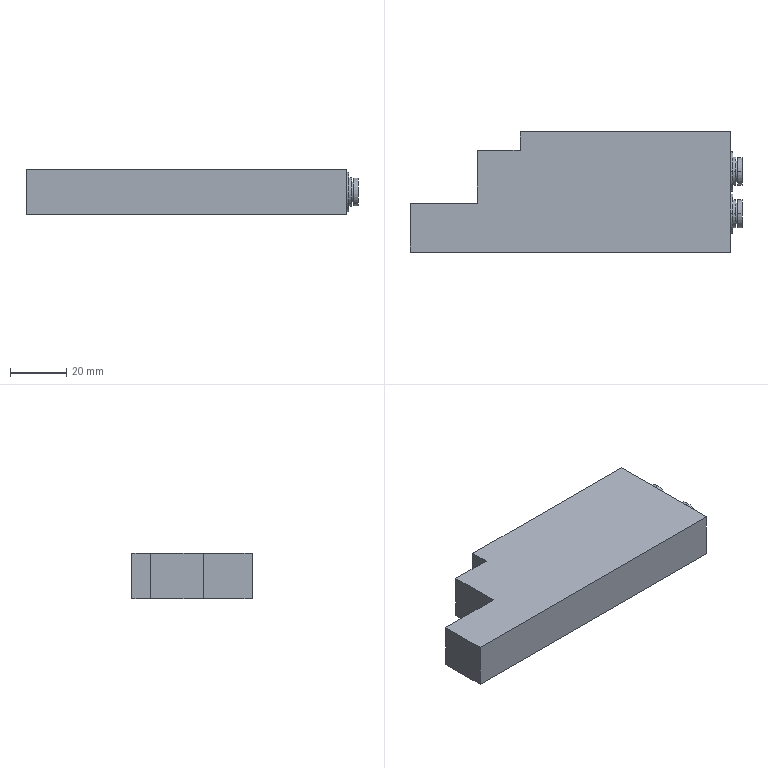Part | SolidWorks | features BaseBody 1 | 1 solid | 116 faces | box 117.6 x 42.6 x 16 mm | volume 66009 mm3 | plane 79 | cylinder 37 | commonest cylinder face diameters 6 x4 7.4 x4 9.9 x4 10 x4 14 x4 0.933 x2